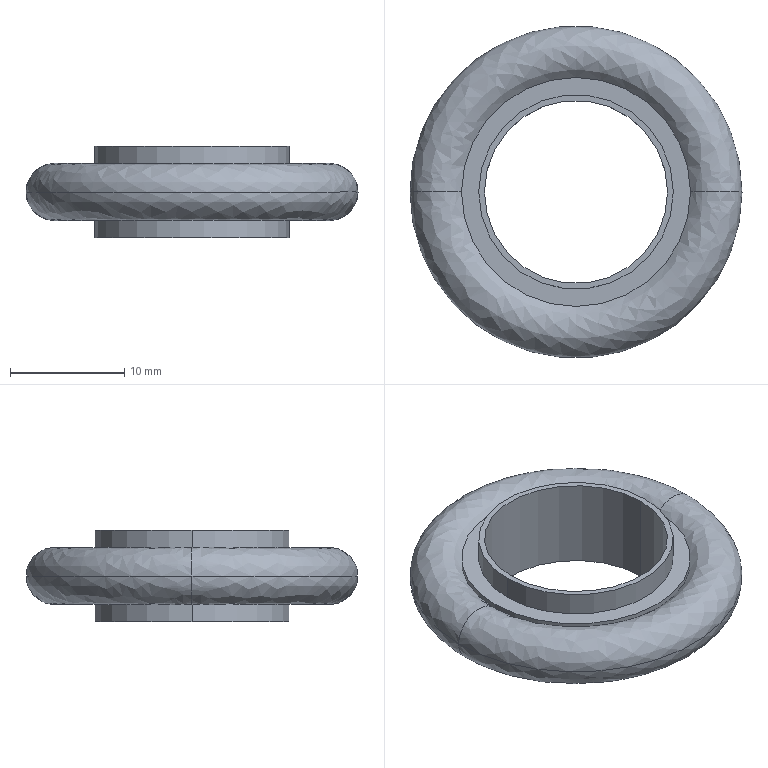Part | SolidWorks | features BaseBody 1 | 1 solid | 18 faces | box 29 x 29 x 8 mm | volume 1965 mm3 | cylinder 10 | spline 4 | plane 4 | commonest cylinder face diameters 17 x4 20 x4 16 x2
STEP:
#1=CARTESIAN_POINT('',(-14.5,0.,0.));
#2=VERTEX_POINT('',#1);
#3=CARTESIAN_POINT('',(14.5,0.,0.));
#4=VERTEX_POINT('',#3);
#5=CARTESIAN_POINT('',(0.,0.,0.));
#6=DIRECTION('',(0.,0.,1.));
#7=DIRECTION('',(1.,0.,0.));
#8=AXIS2_PLACEMENT_3D('',#5,#6,#7);
#9=CIRCLE('',#8,14.5);
#10=EDGE_CURVE('',#2,#4,#9,.T.);
#11=ORIENTED_EDGE('',*,*,#10,.F.);
#12=CARTESIAN_POINT('',(-10.,0.,-1.5));
#13=VERTEX_POINT('',#12);
#14=CARTESIAN_POINT('',(-12.,0.,0.));
#15=DIRECTION('',(0.,-1.,0.));
#16=DIRECTION('',(-1.,0.,0.));
#17=AXIS2_PLACEMENT_3D('',#14,#15,#16);
#18=CIRCLE('',#17,2.5);
#19=EDGE_CURVE('',#2,#13,#18,.T.);
#20=ORIENTED_EDGE('',*,*,#19,.T.);
#21=CARTESIAN_POINT('',(10.,0.,-1.5));
#22=VERTEX_POINT('',#21);
#23=CARTESIAN_POINT('',(0.,0.,-1.5));
#24=DIRECTION('',(0.,0.,1.));
#25=DIRECTION('',(1.,0.,0.));
#26=AXIS2_PLACEMENT_3D('',#23,#24,#25);
#27=CIRCLE('',#26,10.);
#28=EDGE_CURVE('',#13,#22,#27,.T.);
#29=ORIENTED_EDGE('',*,*,#28,.T.);
#30=CARTESIAN_POINT('',(12.,0.,0.));
#31=DIRECTION('',(0.,1.,0.));
#32=DIRECTION('',(1.,0.,0.));
#33=AXIS2_PLACEMENT_3D('',#30,#31,#32);
#34=CIRCLE('',#33,2.5);
#35=EDGE_CURVE('',#4,#22,#34,.T.);
#36=ORIENTED_EDGE('',*,*,#35,.F.);
#37=EDGE_LOOP('',(#11,#20,#29,#36));
#38=FACE_OUTER_BOUND('',#37,.T.);
#39=CARTESIAN_POINT('',(-14.5,0.,0.));
#40=CARTESIAN_POINT('',(-14.5,-29.,0.));
#41=CARTESIAN_POINT('',(14.5,-29.,0.));
#42=CARTESIAN_POINT('',(14.5,0.,0.));
#43=CARTESIAN_POINT('',(-14.5,0.,-2.906));
#44=CARTESIAN_POINT('',(-14.5,-29.,-2.906));
#45=CARTESIAN_POINT('',(14.5,-29.,-2.906));
#46=CARTESIAN_POINT('',(14.5,0.,-2.906));
#47=CARTESIAN_POINT('',(-11.743,0.,-3.825));
#48=CARTESIAN_POINT('',(-11.743,-23.487,-3.825));
#49=CARTESIAN_POINT('',(11.743,-23.487,-3.825));
#50=CARTESIAN_POINT('',(11.743,0.,-3.825));
#51=CARTESIAN_POINT('',(-10.,0.,-1.5));
#52=CARTESIAN_POINT('',(-10.,-20.,-1.5));
#53=CARTESIAN_POINT('',(10.,-20.,-1.5));
#54=CARTESIAN_POINT('',(10.,0.,-1.5));
#55=(BOUNDED_SURFACE()B_SPLINE_SURFACE(3,3,((#39,#40,#41,#42),(#43,#44,#45,#46),(#47,#48,#49,#50),(#51,#52,#53,#54)),.UNSPECIFIED.,.F.,.F.,.T.)B_SPLINE_SURFACE_WITH_KNOTS((4,4),(4,4),(0.,1.),(0.,1.),.UNSPECIFIED.)GEOMETRIC_REPRESENTATION_ITEM()RATIONAL_B_SPLINE_SURFACE(((1.,0.3333,0.3333,1.),(0.5442,0.1814,0.1814,0.5442),(0.5442,0.1814,0.1814,0.5442),(1.,0.3333,0.3333,1.)))REPRESENTATION_ITEM('')SURFACE());
#56=ADVANCED_FACE('',(#38),#55,.T.);
#57=CARTESIAN_POINT('',(10.,0.,1.5));
#58=VERTEX_POINT('',#57);
#59=CARTESIAN_POINT('',(-10.,0.,1.5));
#60=VERTEX_POINT('',#59);
#61=CARTESIAN_POINT('',(0.,0.,1.5));
#62=DIRECTION('',(0.,0.,-1.));
#63=DIRECTION('',(1.,0.,0.));
#64=AXIS2_PLACEMENT_3D('',#61,#62,#63);
#65=CIRCLE('',#64,10.);
#66=EDGE_CURVE('',#58,#60,#65,.T.);
#67=ORIENTED_EDGE('',*,*,#66,.T.);
#68=CARTESIAN_POINT('',(-12.,0.,0.));
#69=DIRECTION('',(0.,-1.,0.));
#70=DIRECTION('',(-1.,0.,0.));
#71=AXIS2_PLACEMENT_3D('',#68,#69,#70);
#72=CIRCLE('',#71,2.5);
#73=EDGE_CURVE('',#60,#2,#72,.T.);
#74=ORIENTED_EDGE('',*,*,#73,.T.);
#75=ORIENTED_EDGE('',*,*,#10,.T.);
#76=CARTESIAN_POINT('',(12.,0.,0.));
#77=DIRECTION('',(0.,1.,0.));
#78=DIRECTION('',(1.,0.,0.));
#79=AXIS2_PLACEMENT_3D('',#76,#77,#78);
#80=CIRCLE('',#79,2.5);
#81=EDGE_CURVE('',#58,#4,#80,.T.);
#82=ORIENTED_EDGE('',*,*,#81,.F.);
#83=EDGE_LOOP('',(#67,#74,#75,#82));
#84=FACE_OUTER_BOUND('',#83,.T.);
#85=CARTESIAN_POINT('',(-10.,0.,1.5));
#86=CARTESIAN_POINT('',(-10.,-20.,1.5));
#87=CARTESIAN_POINT('',(10.,-20.,1.5));
#88=CARTESIAN_POINT('',(10.,0.,1.5));
#89=CARTESIAN_POINT('',(-11.743,0.,3.825));
#90=CARTESIAN_POINT('',(-11.743,-23.487,3.825));
#91=CARTESIAN_POINT('',(11.743,-23.487,3.825));
#92=CARTESIAN_POINT('',(11.743,0.,3.825));
#93=CARTESIAN_POINT('',(-14.5,0.,2.906));
#94=CARTESIAN_POINT('',(-14.5,-29.,2.906));
#95=CARTESIAN_POINT('',(14.5,-29.,2.906));
#96=CARTESIAN_POINT('',(14.5,0.,2.906));
#97=CARTESIAN_POINT('',(-14.5,0.,0.));
#98=CARTESIAN_POINT('',(-14.5,-29.,0.));
#99=CARTESIAN_POINT('',(14.5,-29.,0.));
#100=CARTESIAN_POINT('',(14.5,0.,0.));
#101=(BOUNDED_SURFACE()B_SPLINE_SURFACE(3,3,((#85,#86,#87,#88),(#89,#90,#91,#92),(#93,#94,#95,#96),(#97,#98,#99,#100)),.UNSPECIFIED.,.F.,.F.,.F.)B_SPLINE_SURFACE_WITH_KNOTS((4,4),(4,4),(0.,1.),(0.,1.),.UNSPECIFIED.)GEOMETRIC_REPRESENTATION_ITEM()RATIONAL_B_SPLINE_SURFACE(((1.,0.3333,0.3333,1.),(0.5442,0.1814,0.1814,0.5442),(0.5442,0.1814,0.1814,0.5442),(1.,0.3333,0.3333,1.)))REPRESENTATION_ITEM('')SURFACE());
#102=ADVANCED_FACE('',(#84),#101,.T.);
#103=ORIENTED_EDGE('',*,*,#73,.F.);
#104=CARTESIAN_POINT('',(0.,0.,1.5));
#105=DIRECTION('',(0.,0.,-1.));
#106=DIRECTION('',(1.,0.,0.));
#107=AXIS2_PLACEMENT_3D('',#104,#105,#106);
#108=CIRCLE('',#107,10.);
#109=EDGE_CURVE('',#60,#58,#108,.T.);
#110=ORIENTED_EDGE('',*,*,#109,.T.);
#111=ORIENTED_EDGE('',*,*,#81,.T.);
#112=CARTESIAN_POINT('',(0.,0.,0.));
#113=DIRECTION('',(0.,0.,1.));
#114=DIRECTION('',(1.,0.,0.));
#115=AXIS2_PLACEMENT_3D('',#112,#113,#114);
#116=CIRCLE('',#115,14.5);
#117=EDGE_CURVE('',#4,#2,#116,.T.);
#118=ORIENTED_EDGE('',*,*,#117,.T.);
#119=EDGE_LOOP('',(#103,#110,#111,#118));
#120=FACE_OUTER_BOUND('',#119,.T.);
#121=CARTESIAN_POINT('',(10.,0.,1.5));
#122=CARTESIAN_POINT('',(10.,20.,1.5));
#123=CARTESIAN_POINT('',(-10.,20.,1.5));
#124=CARTESIAN_POINT('',(-10.,0.,1.5));
#125=CARTESIAN_POINT('',(11.743,0.,3.825));
#126=CARTESIAN_POINT('',(11.743,23.487,3.825));
#127=CARTESIAN_POINT('',(-11.743,23.487,3.825));
#128=CARTESIAN_POINT('',(-11.743,0.,3.825));
#129=CARTESIAN_POINT('',(14.5,0.,2.906));
#130=CARTESIAN_POINT('',(14.5,29.,2.906));
#131=CARTESIAN_POINT('',(-14.5,29.,2.906));
#132=CARTESIAN_POINT('',(-14.5,0.,2.906));
#133=CARTESIAN_POINT('',(14.5,0.,0.));
#134=CARTESIAN_POINT('',(14.5,29.,0.));
#135=CARTESIAN_POINT('',(-14.5,29.,0.));
#136=CARTESIAN_POINT('',(-14.5,0.,0.));
#137=(BOUNDED_SURFACE()B_SPLINE_SURFACE(3,3,((#121,#122,#123,#124),(#125,#126,#127,#128),(#129,#130,#131,#132),(#133,#134,#135,#136)),.UNSPECIFIED.,.F.,.F.,.F.)B_SPLINE_SURFACE_WITH_KNOTS((4,4),(4,4),(0.,1.),(0.,1.),.UNSPECIFIED.)GEOMETRIC_REPRESENTATION_ITEM()RATIONAL_B_SPLINE_SURFACE(((1.,0.3333,0.3333,1.),(0.5442,0.1814,0.1814,0.5442),(0.5442,0.1814,0.1814,0.5442),(1.,0.3333,0.3333,1.)))REPRESENTATION_ITEM('')SURFACE());
#138=ADVANCED_FACE('',(#120),#137,.T.);
#139=ORIENTED_EDGE('',*,*,#109,.F.);
#140=CARTESIAN_POINT('',(-10.,0.,1.95));
#141=VERTEX_POINT('',#140);
#142=CARTESIAN_POINT('',(-10.,0.,54.869));
#143=DIRECTION('',(0.,0.,1.));
#144=VECTOR('',#143,1000.);
#145=LINE('',#142,#144);
#146=EDGE_CURVE('',#60,#141,#145,.T.);
#147=ORIENTED_EDGE('',*,*,#146,.T.);
#148=CARTESIAN_POINT('',(10.,0.,1.95));
#149=VERTEX_POINT('',#148);
#150=CARTESIAN_POINT('',(0.,0.,1.95));
#151=DIRECTION('',(0.,0.,-1.));
#152=DIRECTION('',(1.,0.,0.));
#153=AXIS2_PLACEMENT_3D('',#150,#151,#152);
#154=CIRCLE('',#153,10.);
#155=EDGE_CURVE('',#141,#149,#154,.T.);
#156=ORIENTED_EDGE('',*,*,#155,.T.);
#157=CARTESIAN_POINT('',(10.,0.,54.869));
#158=DIRECTION('',(0.,0.,1.));
#159=VECTOR('',#158,1000.);
#160=LINE('',#157,#159);
#161=EDGE_CURVE('',#58,#149,#160,.T.);
#162=ORIENTED_EDGE('',*,*,#161,.F.);
#163=EDGE_LOOP('',(#139,#147,#156,#162));
#164=FACE_OUTER_BOUND('',#163,.T.);
#165=CARTESIAN_POINT('',(0.,0.,54.869));
#166=DIRECTION('',(0.,0.,1.));
#167=DIRECTION('',(1.,0.,0.));
#168=AXIS2_PLACEMENT_3D('',#165,#166,#167);
#169=CYLINDRICAL_SURFACE('',#168,10.);
#170=ADVANCED_FACE('',(#164),#169,.T.);
#171=CARTESIAN_POINT('',(10.,0.,-1.95));
#172=VERTEX_POINT('',#171);
#173=CARTESIAN_POINT('',(-10.,0.,-1.95));
#174=VERTEX_POINT('',#173);
#175=CARTESIAN_POINT('',(0.,0.,-1.95));
#176=DIRECTION('',(0.,0.,1.));
#177=DIRECTION('',(1.,0.,0.));
#178=AXIS2_PLACEMENT_3D('',#175,#176,#177);
#179=CIRCLE('',#178,10.);
#180=EDGE_CURVE('',#172,#174,#179,.T.);
#181=ORIENTED_EDGE('',*,*,#180,.T.);
#182=CARTESIAN_POINT('',(-10.,0.,54.869));
#183=DIRECTION('',(0.,0.,1.));
#184=VECTOR('',#183,1000.);
#185=LINE('',#182,#184);
#186=EDGE_CURVE('',#174,#13,#185,.T.);
#187=ORIENTED_EDGE('',*,*,#186,.T.);
#188=CARTESIAN_POINT('',(0.,0.,-1.5));
#189=DIRECTION('',(0.,0.,1.));
#190=DIRECTION('',(1.,0.,0.));
#191=AXIS2_PLACEMENT_3D('',#188,#189,#190);
#192=CIRCLE('',#191,10.);
#193=EDGE_CURVE('',#22,#13,#192,.T.);
#194=ORIENTED_EDGE('',*,*,#193,.F.);
#195=CARTESIAN_POINT('',(10.,0.,54.869));
#196=DIRECTION('',(0.,0.,1.));
#197=VECTOR('',#196,1000.);
#198=LINE('',#195,#197);
#199=EDGE_CURVE('',#172,#22,#198,.T.);
#200=ORIENTED_EDGE('',*,*,#199,.F.);
#201=EDGE_LOOP('',(#181,#187,#194,#200));
#202=FACE_OUTER_BOUND('',#201,.T.);
#203=CARTESIAN_POINT('',(0.,0.,54.869));
#204=DIRECTION('',(0.,0.,1.));
#205=DIRECTION('',(1.,0.,0.));
#206=AXIS2_PLACEMENT_3D('',#203,#204,#205);
#207=CYLINDRICAL_SURFACE('',#206,10.);
#208=ADVANCED_FACE('',(#202),#207,.T.);
#209=CARTESIAN_POINT('',(8.5,0.,1.95));
#210=VERTEX_POINT('',#209);
#211=CARTESIAN_POINT('',(-8.5,0.,1.95));
#212=VERTEX_POINT('',#211);
#213=CARTESIAN_POINT('',(0.,0.,1.95));
#214=DIRECTION('',(0.,0.,1.));
#215=DIRECTION('',(1.,0.,0.));
#216=AXIS2_PLACEMENT_3D('',#213,#214,#215);
#217=CIRCLE('',#216,8.5);
#218=EDGE_CURVE('',#210,#212,#217,.T.);
#219=ORIENTED_EDGE('',*,*,#218,.T.);
#220=CARTESIAN_POINT('',(-8.5,0.,4.));
#221=VERTEX_POINT('',#220);
#222=CARTESIAN_POINT('',(-8.5,0.,54.869));
#223=DIRECTION('',(0.,0.,1.));
#224=VECTOR('',#223,1000.);
#225=LINE('',#222,#224);
#226=EDGE_CURVE('',#212,#221,#225,.T.);
#227=ORIENTED_EDGE('',*,*,#226,.T.);
#228=CARTESIAN_POINT('',(8.5,0.,4.));
#229=VERTEX_POINT('',#228);
#230=CARTESIAN_POINT('',(0.,0.,4.));
#231=DIRECTION('',(0.,0.,-1.));
#232=DIRECTION('',(1.,0.,0.));
#233=AXIS2_PLACEMENT_3D('',#230,#231,#232);
#234=CIRCLE('',#233,8.5);
#235=EDGE_CURVE('',#221,#229,#234,.T.);
#236=ORIENTED_EDGE('',*,*,#235,.T.);
#237=CARTESIAN_POINT('',(8.5,0.,54.869));
#238=DIRECTION('',(0.,0.,1.));
#239=VECTOR('',#238,1000.);
#240=LINE('',#237,#239);
#241=EDGE_CURVE('',#210,#229,#240,.T.);
#242=ORIENTED_EDGE('',*,*,#241,.F.);
#243=EDGE_LOOP('',(#219,#227,#236,#242));
#244=FACE_OUTER_BOUND('',#243,.T.);
#245=CARTESIAN_POINT('',(0.,0.,54.869));
#246=DIRECTION('',(0.,0.,1.));
#247=DIRECTION('',(1.,0.,0.));
#248=AXIS2_PLACEMENT_3D('',#245,#246,#247);
#249=CYLINDRICAL_SURFACE('',#248,8.5);
#250=ADVANCED_FACE('',(#244),#249,.T.);
#251=CARTESIAN_POINT('',(8.5,0.,-4.));
#252=VERTEX_POINT('',#251);
#253=CARTESIAN_POINT('',(-8.5,0.,-4.));
#254=VERTEX_POINT('',#253);
#255=CARTESIAN_POINT('',(0.,0.,-4.));
#256=DIRECTION('',(0.,0.,1.));
#257=DIRECTION('',(1.,0.,0.));
#258=AXIS2_PLACEMENT_3D('',#255,#256,#257);
#259=CIRCLE('',#258,8.5);
#260=EDGE_CURVE('',#252,#254,#259,.T.);
#261=ORIENTED_EDGE('',*,*,#260,.T.);
#262=CARTESIAN_POINT('',(-8.5,0.,-1.95));
#263=VERTEX_POINT('',#262);
#264=CARTESIAN_POINT('',(-8.5,0.,54.869));
#265=DIRECTION('',(0.,0.,1.));
#266=VECTOR('',#265,1000.);
#267=LINE('',#264,#266);
#268=EDGE_CURVE('',#254,#263,#267,.T.);
#269=ORIENTED_EDGE('',*,*,#268,.T.);
#270=CARTESIAN_POINT('',(8.5,0.,-1.95));
#271=VERTEX_POINT('',#270);
#272=CARTESIAN_POINT('',(0.,0.,-1.95));
#273=DIRECTION('',(0.,0.,-1.));
#274=DIRECTION('',(1.,0.,0.));
#275=AXIS2_PLACEMENT_3D('',#272,#273,#274);
#276=CIRCLE('',#275,8.5);
#277=EDGE_CURVE('',#263,#271,#276,.T.);
#278=ORIENTED_EDGE('',*,*,#277,.T.);
#279=CARTESIAN_POINT('',(8.5,0.,54.869));
#280=DIRECTION('',(0.,0.,1.));
#281=VECTOR('',#280,1000.);
#282=LINE('',#279,#281);
#283=EDGE_CURVE('',#252,#271,#282,.T.);
#284=ORIENTED_EDGE('',*,*,#283,.F.);
#285=EDGE_LOOP('',(#261,#269,#278,#284));
#286=FACE_OUTER_BOUND('',#285,.T.);
#287=CARTESIAN_POINT('',(0.,0.,54.869));
#288=DIRECTION('',(0.,0.,1.));
#289=DIRECTION('',(1.,0.,0.));
#290=AXIS2_PLACEMENT_3D('',#287,#288,#289);
#291=CYLINDRICAL_SURFACE('',#290,8.5);
#292=ADVANCED_FACE('',(#286),#291,.T.);
#293=CARTESIAN_POINT('',(8.,0.,-4.));
#294=VERTEX_POINT('',#293);
#295=CARTESIAN_POINT('',(-8.,0.,-4.));
#296=VERTEX_POINT('',#295);
#297=CARTESIAN_POINT('',(0.,0.,-4.));
#298=DIRECTION('',(0.,0.,-1.));
#299=DIRECTION('',(1.,0.,0.));
#300=AXIS2_PLACEMENT_3D('',#297,#298,#299);
#301=CIRCLE('',#300,8.);
#302=EDGE_CURVE('',#294,#296,#301,.T.);
#303=ORIENTED_EDGE('',*,*,#302,.T.);
#304=CARTESIAN_POINT('',(-8.,0.,4.));
#305=VERTEX_POINT('',#304);
#306=CARTESIAN_POINT('',(-8.,0.,54.869));
#307=DIRECTION('',(0.,0.,1.));
#308=VECTOR('',#307,1000.);
#309=LINE('',#306,#308);
#310=EDGE_CURVE('',#296,#305,#309,.T.);
#311=ORIENTED_EDGE('',*,*,#310,.T.);
#312=CARTESIAN_POINT('',(8.,0.,4.));
#313=VERTEX_POINT('',#312);
#314=CARTESIAN_POINT('',(0.,0.,4.));
#315=DIRECTION('',(0.,0.,1.));
#316=DIRECTION('',(1.,0.,0.));
#317=AXIS2_PLACEMENT_3D('',#314,#315,#316);
#318=CIRCLE('',#317,8.);
#319=EDGE_CURVE('',#305,#313,#318,.T.);
#320=ORIENTED_EDGE('',*,*,#319,.T.);
#321=CARTESIAN_POINT('',(8.,0.,54.869));
#322=DIRECTION('',(0.,0.,1.));
#323=VECTOR('',#322,1000.);
#324=LINE('',#321,#323);
#325=EDGE_CURVE('',#294,#313,#324,.T.);
#326=ORIENTED_EDGE('',*,*,#325,.F.);
#327=EDGE_LOOP('',(#303,#311,#320,#326));
#328=FACE_OUTER_BOUND('',#327,.T.);
#329=CARTESIAN_POINT('',(0.,0.,54.869));
#330=DIRECTION('',(0.,0.,1.));
#331=DIRECTION('',(1.,0.,0.));
#332=AXIS2_PLACEMENT_3D('',#329,#330,#331);
#333=CYLINDRICAL_SURFACE('',#332,8.);
#334=ADVANCED_FACE('',(#328),#333,.F.);
#335=ORIENTED_EDGE('',*,*,#19,.F.);
#336=ORIENTED_EDGE('',*,*,#117,.F.);
#337=ORIENTED_EDGE('',*,*,#35,.T.);
#338=ORIENTED_EDGE('',*,*,#193,.T.);
#339=EDGE_LOOP('',(#335,#336,#337,#338));
#340=FACE_OUTER_BOUND('',#339,.T.);
#341=CARTESIAN_POINT('',(14.5,0.,0.));
#342=CARTESIAN_POINT('',(14.5,29.,0.));
#343=CARTESIAN_POINT('',(-14.5,29.,0.));
#344=CARTESIAN_POINT('',(-14.5,0.,0.));
#345=CARTESIAN_POINT('',(14.5,0.,-2.906));
#346=CARTESIAN_POINT('',(14.5,29.,-2.906));
#347=CARTESIAN_POINT('',(-14.5,29.,-2.906));
#348=CARTESIAN_POINT('',(-14.5,0.,-2.906));
#349=CARTESIAN_POINT('',(11.743,0.,-3.825));
#350=CARTESIAN_POINT('',(11.743,23.487,-3.825));
#351=CARTESIAN_POINT('',(-11.743,23.487,-3.825));
#352=CARTESIAN_POINT('',(-11.743,0.,-3.825));
#353=CARTESIAN_POINT('',(10.,0.,-1.5));
#354=CARTESIAN_POINT('',(10.,20.,-1.5));
#355=CARTESIAN_POINT('',(-10.,20.,-1.5));
#356=CARTESIAN_POINT('',(-10.,0.,-1.5));
#357=(BOUNDED_SURFACE()B_SPLINE_SURFACE(3,3,((#341,#342,#343,#344),(#345,#346,#347,#348),(#349,#350,#351,#352),(#353,#354,#355,#356)),.UNSPECIFIED.,.F.,.F.,.T.)B_SPLINE_SURFACE_WITH_KNOTS((4,4),(4,4),(0.,1.),(0.,1.),.UNSPECIFIED.)GEOMETRIC_REPRESENTATION_ITEM()RATIONAL_B_SPLINE_SURFACE(((1.,0.3333,0.3333,1.),(0.5442,0.1814,0.1814,0.5442),(0.5442,0.1814,0.1814,0.5442),(1.,0.3333,0.3333,1.)))REPRESENTATION_ITEM('')SURFACE());
#358=ADVANCED_FACE('',(#340),#357,.T.);
#359=ORIENTED_EDGE('',*,*,#146,.F.);
#360=ORIENTED_EDGE('',*,*,#66,.F.);
#361=ORIENTED_EDGE('',*,*,#161,.T.);
#362=CARTESIAN_POINT('',(0.,0.,1.95));
#363=DIRECTION('',(0.,0.,-1.));
#364=DIRECTION('',(1.,0.,0.));
#365=AXIS2_PLACEMENT_3D('',#362,#363,#364);
#366=CIRCLE('',#365,10.);
#367=EDGE_CURVE('',#149,#141,#366,.T.);
#368=ORIENTED_EDGE('',*,*,#367,.T.);
#369=EDGE_LOOP('',(#359,#360,#361,#368));
#370=FACE_OUTER_BOUND('',#369,.T.);
#371=CARTESIAN_POINT('',(0.,0.,54.869));
#372=DIRECTION('',(0.,0.,1.));
#373=DIRECTION('',(1.,0.,0.));
#374=AXIS2_PLACEMENT_3D('',#371,#372,#373);
#375=CYLINDRICAL_SURFACE('',#374,10.);
#376=ADVANCED_FACE('',(#370),#375,.T.);
#377=ORIENTED_EDGE('',*,*,#186,.F.);
#378=CARTESIAN_POINT('',(0.,0.,-1.95));
#379=DIRECTION('',(0.,0.,1.));
#380=DIRECTION('',(1.,0.,0.));
#381=AXIS2_PLACEMENT_3D('',#378,#379,#380);
#382=CIRCLE('',#381,10.);
#383=EDGE_CURVE('',#174,#172,#382,.T.);
#384=ORIENTED_EDGE('',*,*,#383,.T.);
#385=ORIENTED_EDGE('',*,*,#199,.T.);
#386=ORIENTED_EDGE('',*,*,#28,.F.);
#387=EDGE_LOOP('',(#377,#384,#385,#386));
#388=FACE_OUTER_BOUND('',#387,.T.);
#389=CARTESIAN_POINT('',(0.,0.,54.869));
#390=DIRECTION('',(0.,0.,1.));
#391=DIRECTION('',(1.,0.,0.));
#392=AXIS2_PLACEMENT_3D('',#389,#390,#391);
#393=CYLINDRICAL_SURFACE('',#392,10.);
#394=ADVANCED_FACE('',(#388),#393,.T.);
#395=ORIENTED_EDGE('',*,*,#367,.F.);
#396=ORIENTED_EDGE('',*,*,#155,.F.);
#397=EDGE_LOOP('',(#395,#396));
#398=FACE_OUTER_BOUND('',#397,.T.);
#399=ORIENTED_EDGE('',*,*,#218,.F.);
#400=CARTESIAN_POINT('',(0.,0.,1.95));
#401=DIRECTION('',(0.,0.,1.));
#402=DIRECTION('',(1.,0.,0.));
#403=AXIS2_PLACEMENT_3D('',#400,#401,#402);
#404=CIRCLE('',#403,8.5);
#405=EDGE_CURVE('',#212,#210,#404,.T.);
#406=ORIENTED_EDGE('',*,*,#405,.F.);
#407=EDGE_LOOP('',(#399,#406));
#408=FACE_BOUND('',#407,.T.);
#409=CARTESIAN_POINT('',(10.,0.,1.95));
#410=DIRECTION('',(0.,0.,-1.));
#411=DIRECTION('',(-1.,0.,0.));
#412=AXIS2_PLACEMENT_3D('',#409,#410,#411);
#413=PLANE('',#412);
#414=ADVANCED_FACE('',(#398,#408),#413,.F.);
#415=CARTESIAN_POINT('',(0.,0.,-1.95));
#416=DIRECTION('',(0.,0.,-1.));
#417=DIRECTION('',(1.,0.,0.));
#418=AXIS2_PLACEMENT_3D('',#415,#416,#417);
#419=CIRCLE('',#418,8.5);
#420=EDGE_CURVE('',#271,#263,#419,.T.);
#421=ORIENTED_EDGE('',*,*,#420,.F.);
#422=ORIENTED_EDGE('',*,*,#277,.F.);
#423=EDGE_LOOP('',(#421,#422));
#424=FACE_BOUND('',#423,.T.);
#425=ORIENTED_EDGE('',*,*,#180,.F.);
#426=ORIENTED_EDGE('',*,*,#383,.F.);
#427=EDGE_LOOP('',(#425,#426));
#428=FACE_OUTER_BOUND('',#427,.T.);
#429=CARTESIAN_POINT('',(8.5,0.,-1.95));
#430=DIRECTION('',(0.,0.,1.));
#431=DIRECTION('',(1.,0.,0.));
#432=AXIS2_PLACEMENT_3D('',#429,#430,#431);
#433=PLANE('',#432);
#434=ADVANCED_FACE('',(#424,#428),#433,.F.);
#435=ORIENTED_EDGE('',*,*,#226,.F.);
#436=ORIENTED_EDGE('',*,*,#405,.T.);
#437=ORIENTED_EDGE('',*,*,#241,.T.);
#438=CARTESIAN_POINT('',(0.,0.,4.));
#439=DIRECTION('',(0.,0.,-1.));
#440=DIRECTION('',(1.,0.,0.));
#441=AXIS2_PLACEMENT_3D('',#438,#439,#440);
#442=CIRCLE('',#441,8.5);
#443=EDGE_CURVE('',#229,#221,#442,.T.);
#444=ORIENTED_EDGE('',*,*,#443,.T.);
#445=EDGE_LOOP('',(#435,#436,#437,#444));
#446=FACE_OUTER_BOUND('',#445,.T.);
#447=CARTESIAN_POINT('',(0.,0.,54.869));
#448=DIRECTION('',(0.,0.,1.));
#449=DIRECTION('',(1.,0.,0.));
#450=AXIS2_PLACEMENT_3D('',#447,#448,#449);
#451=CYLINDRICAL_SURFACE('',#450,8.5);
#452=ADVANCED_FACE('',(#446),#451,.T.);
#453=ORIENTED_EDGE('',*,*,#268,.F.);
#454=CARTESIAN_POINT('',(0.,0.,-4.));
#455=DIRECTION('',(0.,0.,1.));
#456=DIRECTION('',(1.,0.,0.));
#457=AXIS2_PLACEMENT_3D('',#454,#455,#456);
#458=CIRCLE('',#457,8.5);
#459=EDGE_CURVE('',#254,#252,#458,.T.);
#460=ORIENTED_EDGE('',*,*,#459,.T.);
#461=ORIENTED_EDGE('',*,*,#283,.T.);
#462=ORIENTED_EDGE('',*,*,#420,.T.);
#463=EDGE_LOOP('',(#453,#460,#461,#462));
#464=FACE_OUTER_BOUND('',#463,.T.);
#465=CARTESIAN_POINT('',(0.,0.,54.869));
#466=DIRECTION('',(0.,0.,1.));
#467=DIRECTION('',(1.,0.,0.));
#468=AXIS2_PLACEMENT_3D('',#465,#466,#467);
#469=CYLINDRICAL_SURFACE('',#468,8.5);
#470=ADVANCED_FACE('',(#464),#469,.T.);
#471=ORIENTED_EDGE('',*,*,#443,.F.);
#472=ORIENTED_EDGE('',*,*,#235,.F.);
#473=EDGE_LOOP('',(#471,#472));
#474=FACE_OUTER_BOUND('',#473,.T.);
#475=CARTESIAN_POINT('',(0.,0.,4.));
#476=DIRECTION('',(0.,0.,1.));
#477=DIRECTION('',(1.,0.,0.));
#478=AXIS2_PLACEMENT_3D('',#475,#476,#477);
#479=CIRCLE('',#478,8.);
#480=EDGE_CURVE('',#313,#305,#479,.T.);
#481=ORIENTED_EDGE('',*,*,#480,.F.);
#482=ORIENTED_EDGE('',*,*,#319,.F.);
#483=EDGE_LOOP('',(#481,#482));
#484=FACE_BOUND('',#483,.T.);
#485=CARTESIAN_POINT('',(8.5,0.,4.));
#486=DIRECTION('',(0.,0.,-1.));
#487=DIRECTION('',(-1.,0.,0.));
#488=AXIS2_PLACEMENT_3D('',#485,#486,#487);
#489=PLANE('',#488);
#490=ADVANCED_FACE('',(#474,#484),#489,.F.);
#491=ORIENTED_EDGE('',*,*,#302,.F.);
#492=CARTESIAN_POINT('',(0.,0.,-4.));
#493=DIRECTION('',(0.,0.,-1.));
#494=DIRECTION('',(1.,0.,0.));
#495=AXIS2_PLACEMENT_3D('',#492,#493,#494);
#496=CIRCLE('',#495,8.);
#497=EDGE_CURVE('',#296,#294,#496,.T.);
#498=ORIENTED_EDGE('',*,*,#497,.F.);
#499=EDGE_LOOP('',(#491,#498));
#500=FACE_BOUND('',#499,.T.);
#501=ORIENTED_EDGE('',*,*,#260,.F.);
#502=ORIENTED_EDGE('',*,*,#459,.F.);
#503=EDGE_LOOP('',(#501,#502));
#504=FACE_OUTER_BOUND('',#503,.T.);
#505=CARTESIAN_POINT('',(8.,0.,-4.));
#506=DIRECTION('',(0.,0.,1.));
#507=DIRECTION('',(1.,0.,0.));
#508=AXIS2_PLACEMENT_3D('',#505,#506,#507);
#509=PLANE('',#508);
#510=ADVANCED_FACE('',(#500,#504),#509,.F.);
#511=ORIENTED_EDGE('',*,*,#310,.F.);
#512=ORIENTED_EDGE('',*,*,#497,.T.);
#513=ORIENTED_EDGE('',*,*,#325,.T.);
#514=ORIENTED_EDGE('',*,*,#480,.T.);
#515=EDGE_LOOP('',(#511,#512,#513,#514));
#516=FACE_OUTER_BOUND('',#515,.T.);
#517=CARTESIAN_POINT('',(0.,0.,54.869));
#518=DIRECTION('',(0.,0.,1.));
#519=DIRECTION('',(1.,0.,0.));
#520=AXIS2_PLACEMENT_3D('',#517,#518,#519);
#521=CYLINDRICAL_SURFACE('',#520,8.);
#522=ADVANCED_FACE('',(#516),#521,.F.);
#523=CLOSED_SHELL('',(#56,#102,#138,#170,#208,#250,#292,#334,#358,#376,#394,#414,#434,#452,#470,#490,#510,#522));
#524=MANIFOLD_SOLID_BREP('',#523);
#525=CARTESIAN_POINT('',(0.,0.,0.));
#526=DIRECTION('',(0.,0.,1.));
#527=DIRECTION('',(1.,0.,0.));
#528=AXIS2_PLACEMENT_3D('',#525,#526,#527);
#529=(LENGTH_UNIT()NAMED_UNIT(*)SI_UNIT(.MILLI.,.METRE.));
#530=UNCERTAINTY_MEASURE_WITH_UNIT(LENGTH_MEASURE(0.00001),#529,'','');
#531=(NAMED_UNIT(*)PLANE_ANGLE_UNIT()SI_UNIT($,.RADIAN.));
#532=(NAMED_UNIT(*)SI_UNIT($,.STERADIAN.)SOLID_ANGLE_UNIT());
#533=(GEOMETRIC_REPRESENTATION_CONTEXT(3)GLOBAL_UNCERTAINTY_ASSIGNED_CONTEXT((#530))GLOBAL_UNIT_ASSIGNED_CONTEXT((#529,#531,#532))REPRESENTATION_CONTEXT('',''));
#534=ADVANCED_BREP_SHAPE_REPRESENTATION('',(#524,#528),#533);